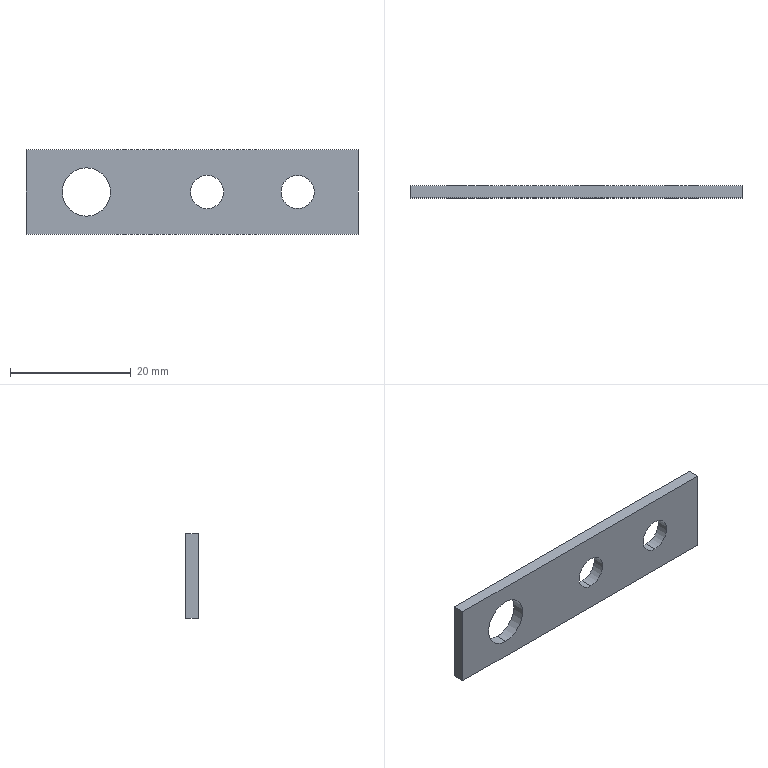Part | SolidWorks | features RefAxis 3, 3DProfileFeature 1, Extrusion 1 | 1 solid | 12 faces | box 55 x 2 x 14 mm | volume 1344 mm3 | cylinder 6 | plane 6 | commonest cylinder face diameters 5.5 x4 8 x2
STEP:
#1=CARTESIAN_POINT('',(0.,1.,-4.));
#2=VERTEX_POINT('',#1);
#3=CARTESIAN_POINT('',(0.,1.,4.));
#4=VERTEX_POINT('',#3);
#5=CARTESIAN_POINT('',(0.,1.,0.));
#6=DIRECTION('',(0.,1.,0.));
#7=DIRECTION('',(0.,0.,1.));
#8=AXIS2_PLACEMENT_3D('',#5,#6,#7);
#9=CIRCLE('',#8,4.);
#10=EDGE_CURVE('',#2,#4,#9,.T.);
#11=ORIENTED_EDGE('',*,*,#10,.T.);
#12=CARTESIAN_POINT('',(0.,-1.,4.));
#13=VERTEX_POINT('',#12);
#14=CARTESIAN_POINT('',(0.,1.,4.));
#15=DIRECTION('',(0.,-1.,0.));
#16=VECTOR('',#15,1000.);
#17=LINE('',#14,#16);
#18=EDGE_CURVE('',#4,#13,#17,.T.);
#19=ORIENTED_EDGE('',*,*,#18,.T.);
#20=CARTESIAN_POINT('',(0.,-1.,-4.));
#21=VERTEX_POINT('',#20);
#22=CARTESIAN_POINT('',(0.,-1.,0.));
#23=DIRECTION('',(0.,1.,0.));
#24=DIRECTION('',(0.,0.,1.));
#25=AXIS2_PLACEMENT_3D('',#22,#23,#24);
#26=CIRCLE('',#25,4.);
#27=EDGE_CURVE('',#21,#13,#26,.T.);
#28=ORIENTED_EDGE('',*,*,#27,.F.);
#29=CARTESIAN_POINT('',(0.,1.,-4.));
#30=DIRECTION('',(0.,-1.,0.));
#31=VECTOR('',#30,1000.);
#32=LINE('',#29,#31);
#33=EDGE_CURVE('',#2,#21,#32,.T.);
#34=ORIENTED_EDGE('',*,*,#33,.F.);
#35=EDGE_LOOP('',(#11,#19,#28,#34));
#36=FACE_OUTER_BOUND('',#35,.T.);
#37=CARTESIAN_POINT('',(0.,1.,0.));
#38=DIRECTION('',(0.,-1.,0.));
#39=DIRECTION('',(0.,0.,-1.));
#40=AXIS2_PLACEMENT_3D('',#37,#38,#39);
#41=CYLINDRICAL_SURFACE('',#40,4.);
#42=ADVANCED_FACE('',(#36),#41,.F.);
#43=CARTESIAN_POINT('',(20.,1.,-2.75));
#44=VERTEX_POINT('',#43);
#45=CARTESIAN_POINT('',(20.,1.,2.75));
#46=VERTEX_POINT('',#45);
#47=CARTESIAN_POINT('',(20.,1.,0.));
#48=DIRECTION('',(0.,1.,0.));
#49=DIRECTION('',(0.,0.,1.));
#50=AXIS2_PLACEMENT_3D('',#47,#48,#49);
#51=CIRCLE('',#50,2.75);
#52=EDGE_CURVE('',#44,#46,#51,.T.);
#53=ORIENTED_EDGE('',*,*,#52,.T.);
#54=CARTESIAN_POINT('',(20.,-1.,2.75));
#55=VERTEX_POINT('',#54);
#56=CARTESIAN_POINT('',(20.,1.,2.75));
#57=DIRECTION('',(0.,-1.,0.));
#58=VECTOR('',#57,1000.);
#59=LINE('',#56,#58);
#60=EDGE_CURVE('',#46,#55,#59,.T.);
#61=ORIENTED_EDGE('',*,*,#60,.T.);
#62=CARTESIAN_POINT('',(20.,-1.,-2.75));
#63=VERTEX_POINT('',#62);
#64=CARTESIAN_POINT('',(20.,-1.,0.));
#65=DIRECTION('',(0.,1.,0.));
#66=DIRECTION('',(0.,0.,1.));
#67=AXIS2_PLACEMENT_3D('',#64,#65,#66);
#68=CIRCLE('',#67,2.75);
#69=EDGE_CURVE('',#63,#55,#68,.T.);
#70=ORIENTED_EDGE('',*,*,#69,.F.);
#71=CARTESIAN_POINT('',(20.,1.,-2.75));
#72=DIRECTION('',(0.,-1.,0.));
#73=VECTOR('',#72,1000.);
#74=LINE('',#71,#73);
#75=EDGE_CURVE('',#44,#63,#74,.T.);
#76=ORIENTED_EDGE('',*,*,#75,.F.);
#77=EDGE_LOOP('',(#53,#61,#70,#76));
#78=FACE_OUTER_BOUND('',#77,.T.);
#79=CARTESIAN_POINT('',(20.,1.,0.));
#80=DIRECTION('',(0.,-1.,0.));
#81=DIRECTION('',(0.,0.,-1.));
#82=AXIS2_PLACEMENT_3D('',#79,#80,#81);
#83=CYLINDRICAL_SURFACE('',#82,2.75);
#84=ADVANCED_FACE('',(#78),#83,.F.);
#85=CARTESIAN_POINT('',(35.,1.,-2.75));
#86=VERTEX_POINT('',#85);
#87=CARTESIAN_POINT('',(35.,1.,2.75));
#88=VERTEX_POINT('',#87);
#89=CARTESIAN_POINT('',(35.,1.,0.));
#90=DIRECTION('',(0.,1.,0.));
#91=DIRECTION('',(0.,0.,1.));
#92=AXIS2_PLACEMENT_3D('',#89,#90,#91);
#93=CIRCLE('',#92,2.75);
#94=EDGE_CURVE('',#86,#88,#93,.T.);
#95=ORIENTED_EDGE('',*,*,#94,.T.);
#96=CARTESIAN_POINT('',(35.,-1.,2.75));
#97=VERTEX_POINT('',#96);
#98=CARTESIAN_POINT('',(35.,1.,2.75));
#99=DIRECTION('',(0.,-1.,0.));
#100=VECTOR('',#99,1000.);
#101=LINE('',#98,#100);
#102=EDGE_CURVE('',#88,#97,#101,.T.);
#103=ORIENTED_EDGE('',*,*,#102,.T.);
#104=CARTESIAN_POINT('',(35.,-1.,-2.75));
#105=VERTEX_POINT('',#104);
#106=CARTESIAN_POINT('',(35.,-1.,0.));
#107=DIRECTION('',(0.,1.,0.));
#108=DIRECTION('',(0.,0.,1.));
#109=AXIS2_PLACEMENT_3D('',#106,#107,#108);
#110=CIRCLE('',#109,2.75);
#111=EDGE_CURVE('',#105,#97,#110,.T.);
#112=ORIENTED_EDGE('',*,*,#111,.F.);
#113=CARTESIAN_POINT('',(35.,1.,-2.75));
#114=DIRECTION('',(0.,-1.,0.));
#115=VECTOR('',#114,1000.);
#116=LINE('',#113,#115);
#117=EDGE_CURVE('',#86,#105,#116,.T.);
#118=ORIENTED_EDGE('',*,*,#117,.F.);
#119=EDGE_LOOP('',(#95,#103,#112,#118));
#120=FACE_OUTER_BOUND('',#119,.T.);
#121=CARTESIAN_POINT('',(35.,1.,0.));
#122=DIRECTION('',(0.,-1.,0.));
#123=DIRECTION('',(0.,0.,-1.));
#124=AXIS2_PLACEMENT_3D('',#121,#122,#123);
#125=CYLINDRICAL_SURFACE('',#124,2.75);
#126=ADVANCED_FACE('',(#120),#125,.F.);
#127=ORIENTED_EDGE('',*,*,#52,.F.);
#128=CARTESIAN_POINT('',(20.,1.,0.));
#129=DIRECTION('',(0.,1.,0.));
#130=DIRECTION('',(0.,0.,1.));
#131=AXIS2_PLACEMENT_3D('',#128,#129,#130);
#132=CIRCLE('',#131,2.75);
#133=EDGE_CURVE('',#46,#44,#132,.T.);
#134=ORIENTED_EDGE('',*,*,#133,.F.);
#135=EDGE_LOOP('',(#127,#134));
#136=FACE_BOUND('',#135,.T.);
#137=CARTESIAN_POINT('',(45.,1.,-7.));
#138=VERTEX_POINT('',#137);
#139=CARTESIAN_POINT('',(-10.,1.,-7.));
#140=VERTEX_POINT('',#139);
#141=CARTESIAN_POINT('',(45.,1.,-7.));
#142=DIRECTION('',(-1.,0.,0.));
#143=VECTOR('',#142,1000.);
#144=LINE('',#141,#143);
#145=EDGE_CURVE('',#138,#140,#144,.T.);
#146=ORIENTED_EDGE('',*,*,#145,.T.);
#147=CARTESIAN_POINT('',(-10.,1.,7.));
#148=VERTEX_POINT('',#147);
#149=CARTESIAN_POINT('',(-10.,1.,-7.));
#150=DIRECTION('',(0.,0.,1.));
#151=VECTOR('',#150,1000.);
#152=LINE('',#149,#151);
#153=EDGE_CURVE('',#140,#148,#152,.T.);
#154=ORIENTED_EDGE('',*,*,#153,.T.);
#155=CARTESIAN_POINT('',(45.,1.,7.));
#156=VERTEX_POINT('',#155);
#157=CARTESIAN_POINT('',(-10.,1.,7.));
#158=DIRECTION('',(1.,0.,0.));
#159=VECTOR('',#158,1000.);
#160=LINE('',#157,#159);
#161=EDGE_CURVE('',#148,#156,#160,.T.);
#162=ORIENTED_EDGE('',*,*,#161,.T.);
#163=CARTESIAN_POINT('',(45.,1.,7.));
#164=DIRECTION('',(0.,0.,-1.));
#165=VECTOR('',#164,1000.);
#166=LINE('',#163,#165);
#167=EDGE_CURVE('',#156,#138,#166,.T.);
#168=ORIENTED_EDGE('',*,*,#167,.T.);
#169=EDGE_LOOP('',(#146,#154,#162,#168));
#170=FACE_OUTER_BOUND('',#169,.T.);
#171=ORIENTED_EDGE('',*,*,#94,.F.);
#172=CARTESIAN_POINT('',(35.,1.,0.));
#173=DIRECTION('',(0.,1.,0.));
#174=DIRECTION('',(0.,0.,1.));
#175=AXIS2_PLACEMENT_3D('',#172,#173,#174);
#176=CIRCLE('',#175,2.75);
#177=EDGE_CURVE('',#88,#86,#176,.T.);
#178=ORIENTED_EDGE('',*,*,#177,.F.);
#179=EDGE_LOOP('',(#171,#178));
#180=FACE_BOUND('',#179,.T.);
#181=ORIENTED_EDGE('',*,*,#10,.F.);
#182=CARTESIAN_POINT('',(0.,1.,0.));
#183=DIRECTION('',(0.,1.,0.));
#184=DIRECTION('',(0.,0.,1.));
#185=AXIS2_PLACEMENT_3D('',#182,#183,#184);
#186=CIRCLE('',#185,4.);
#187=EDGE_CURVE('',#4,#2,#186,.T.);
#188=ORIENTED_EDGE('',*,*,#187,.F.);
#189=EDGE_LOOP('',(#181,#188));
#190=FACE_BOUND('',#189,.T.);
#191=CARTESIAN_POINT('',(0.,1.,0.));
#192=DIRECTION('',(0.,1.,0.));
#193=DIRECTION('',(0.,0.,1.));
#194=AXIS2_PLACEMENT_3D('',#191,#192,#193);
#195=PLANE('',#194);
#196=ADVANCED_FACE('',(#136,#170,#180,#190),#195,.T.);
#197=CARTESIAN_POINT('',(45.,-1.,-7.));
#198=VERTEX_POINT('',#197);
#199=CARTESIAN_POINT('',(45.,1.,-7.));
#200=DIRECTION('',(0.,-1.,0.));
#201=VECTOR('',#200,1000.);
#202=LINE('',#199,#201);
#203=EDGE_CURVE('',#138,#198,#202,.T.);
#204=ORIENTED_EDGE('',*,*,#203,.T.);
#205=CARTESIAN_POINT('',(-10.,-1.,-7.));
#206=VERTEX_POINT('',#205);
#207=CARTESIAN_POINT('',(45.,-1.,-7.));
#208=DIRECTION('',(-1.,0.,0.));
#209=VECTOR('',#208,1000.);
#210=LINE('',#207,#209);
#211=EDGE_CURVE('',#198,#206,#210,.T.);
#212=ORIENTED_EDGE('',*,*,#211,.T.);
#213=CARTESIAN_POINT('',(-10.,1.,-7.));
#214=DIRECTION('',(0.,-1.,0.));
#215=VECTOR('',#214,1000.);
#216=LINE('',#213,#215);
#217=EDGE_CURVE('',#140,#206,#216,.T.);
#218=ORIENTED_EDGE('',*,*,#217,.F.);
#219=ORIENTED_EDGE('',*,*,#145,.F.);
#220=EDGE_LOOP('',(#204,#212,#218,#219));
#221=FACE_OUTER_BOUND('',#220,.T.);
#222=CARTESIAN_POINT('',(45.,1.,-7.));
#223=DIRECTION('',(0.,0.,1.));
#224=DIRECTION('',(1.,0.,0.));
#225=AXIS2_PLACEMENT_3D('',#222,#223,#224);
#226=PLANE('',#225);
#227=ADVANCED_FACE('',(#221),#226,.F.);
#228=ORIENTED_EDGE('',*,*,#217,.T.);
#229=CARTESIAN_POINT('',(-10.,-1.,7.));
#230=VERTEX_POINT('',#229);
#231=CARTESIAN_POINT('',(-10.,-1.,-7.));
#232=DIRECTION('',(0.,0.,1.));
#233=VECTOR('',#232,1000.);
#234=LINE('',#231,#233);
#235=EDGE_CURVE('',#206,#230,#234,.T.);
#236=ORIENTED_EDGE('',*,*,#235,.T.);
#237=CARTESIAN_POINT('',(-10.,1.,7.));
#238=DIRECTION('',(0.,-1.,0.));
#239=VECTOR('',#238,1000.);
#240=LINE('',#237,#239);
#241=EDGE_CURVE('',#148,#230,#240,.T.);
#242=ORIENTED_EDGE('',*,*,#241,.F.);
#243=ORIENTED_EDGE('',*,*,#153,.F.);
#244=EDGE_LOOP('',(#228,#236,#242,#243));
#245=FACE_OUTER_BOUND('',#244,.T.);
#246=CARTESIAN_POINT('',(-10.,1.,-7.));
#247=DIRECTION('',(1.,0.,0.));
#248=DIRECTION('',(0.,0.,-1.));
#249=AXIS2_PLACEMENT_3D('',#246,#247,#248);
#250=PLANE('',#249);
#251=ADVANCED_FACE('',(#245),#250,.F.);
#252=ORIENTED_EDGE('',*,*,#241,.T.);
#253=CARTESIAN_POINT('',(45.,-1.,7.));
#254=VERTEX_POINT('',#253);
#255=CARTESIAN_POINT('',(-10.,-1.,7.));
#256=DIRECTION('',(1.,0.,0.));
#257=VECTOR('',#256,1000.);
#258=LINE('',#255,#257);
#259=EDGE_CURVE('',#230,#254,#258,.T.);
#260=ORIENTED_EDGE('',*,*,#259,.T.);
#261=CARTESIAN_POINT('',(45.,1.,7.));
#262=DIRECTION('',(0.,-1.,0.));
#263=VECTOR('',#262,1000.);
#264=LINE('',#261,#263);
#265=EDGE_CURVE('',#156,#254,#264,.T.);
#266=ORIENTED_EDGE('',*,*,#265,.F.);
#267=ORIENTED_EDGE('',*,*,#161,.F.);
#268=EDGE_LOOP('',(#252,#260,#266,#267));
#269=FACE_OUTER_BOUND('',#268,.T.);
#270=CARTESIAN_POINT('',(-10.,1.,7.));
#271=DIRECTION('',(0.,0.,-1.));
#272=DIRECTION('',(-1.,0.,0.));
#273=AXIS2_PLACEMENT_3D('',#270,#271,#272);
#274=PLANE('',#273);
#275=ADVANCED_FACE('',(#269),#274,.F.);
#276=ORIENTED_EDGE('',*,*,#265,.T.);
#277=CARTESIAN_POINT('',(45.,-1.,7.));
#278=DIRECTION('',(0.,0.,-1.));
#279=VECTOR('',#278,1000.);
#280=LINE('',#277,#279);
#281=EDGE_CURVE('',#254,#198,#280,.T.);
#282=ORIENTED_EDGE('',*,*,#281,.T.);
#283=ORIENTED_EDGE('',*,*,#203,.F.);
#284=ORIENTED_EDGE('',*,*,#167,.F.);
#285=EDGE_LOOP('',(#276,#282,#283,#284));
#286=FACE_OUTER_BOUND('',#285,.T.);
#287=CARTESIAN_POINT('',(45.,1.,7.));
#288=DIRECTION('',(-1.,0.,0.));
#289=DIRECTION('',(0.,0.,1.));
#290=AXIS2_PLACEMENT_3D('',#287,#288,#289);
#291=PLANE('',#290);
#292=ADVANCED_FACE('',(#286),#291,.F.);
#293=ORIENTED_EDGE('',*,*,#102,.F.);
#294=ORIENTED_EDGE('',*,*,#177,.T.);
#295=ORIENTED_EDGE('',*,*,#117,.T.);
#296=CARTESIAN_POINT('',(35.,-1.,0.));
#297=DIRECTION('',(0.,1.,0.));
#298=DIRECTION('',(0.,0.,1.));
#299=AXIS2_PLACEMENT_3D('',#296,#297,#298);
#300=CIRCLE('',#299,2.75);
#301=EDGE_CURVE('',#97,#105,#300,.T.);
#302=ORIENTED_EDGE('',*,*,#301,.F.);
#303=EDGE_LOOP('',(#293,#294,#295,#302));
#304=FACE_OUTER_BOUND('',#303,.T.);
#305=CARTESIAN_POINT('',(35.,1.,0.));
#306=DIRECTION('',(0.,-1.,0.));
#307=DIRECTION('',(0.,0.,-1.));
#308=AXIS2_PLACEMENT_3D('',#305,#306,#307);
#309=CYLINDRICAL_SURFACE('',#308,2.75);
#310=ADVANCED_FACE('',(#304),#309,.F.);
#311=ORIENTED_EDGE('',*,*,#60,.F.);
#312=ORIENTED_EDGE('',*,*,#133,.T.);
#313=ORIENTED_EDGE('',*,*,#75,.T.);
#314=CARTESIAN_POINT('',(20.,-1.,0.));
#315=DIRECTION('',(0.,1.,0.));
#316=DIRECTION('',(0.,0.,1.));
#317=AXIS2_PLACEMENT_3D('',#314,#315,#316);
#318=CIRCLE('',#317,2.75);
#319=EDGE_CURVE('',#55,#63,#318,.T.);
#320=ORIENTED_EDGE('',*,*,#319,.F.);
#321=EDGE_LOOP('',(#311,#312,#313,#320));
#322=FACE_OUTER_BOUND('',#321,.T.);
#323=CARTESIAN_POINT('',(20.,1.,0.));
#324=DIRECTION('',(0.,-1.,0.));
#325=DIRECTION('',(0.,0.,-1.));
#326=AXIS2_PLACEMENT_3D('',#323,#324,#325);
#327=CYLINDRICAL_SURFACE('',#326,2.75);
#328=ADVANCED_FACE('',(#322),#327,.F.);
#329=ORIENTED_EDGE('',*,*,#18,.F.);
#330=ORIENTED_EDGE('',*,*,#187,.T.);
#331=ORIENTED_EDGE('',*,*,#33,.T.);
#332=CARTESIAN_POINT('',(0.,-1.,0.));
#333=DIRECTION('',(0.,1.,0.));
#334=DIRECTION('',(0.,0.,1.));
#335=AXIS2_PLACEMENT_3D('',#332,#333,#334);
#336=CIRCLE('',#335,4.);
#337=EDGE_CURVE('',#13,#21,#336,.T.);
#338=ORIENTED_EDGE('',*,*,#337,.F.);
#339=EDGE_LOOP('',(#329,#330,#331,#338));
#340=FACE_OUTER_BOUND('',#339,.T.);
#341=CARTESIAN_POINT('',(0.,1.,0.));
#342=DIRECTION('',(0.,-1.,0.));
#343=DIRECTION('',(0.,0.,-1.));
#344=AXIS2_PLACEMENT_3D('',#341,#342,#343);
#345=CYLINDRICAL_SURFACE('',#344,4.);
#346=ADVANCED_FACE('',(#340),#345,.F.);
#347=ORIENTED_EDGE('',*,*,#27,.T.);
#348=ORIENTED_EDGE('',*,*,#337,.T.);
#349=EDGE_LOOP('',(#347,#348));
#350=FACE_BOUND('',#349,.T.);
#351=ORIENTED_EDGE('',*,*,#69,.T.);
#352=ORIENTED_EDGE('',*,*,#319,.T.);
#353=EDGE_LOOP('',(#351,#352));
#354=FACE_BOUND('',#353,.T.);
#355=ORIENTED_EDGE('',*,*,#111,.T.);
#356=ORIENTED_EDGE('',*,*,#301,.T.);
#357=EDGE_LOOP('',(#355,#356));
#358=FACE_BOUND('',#357,.T.);
#359=ORIENTED_EDGE('',*,*,#211,.F.);
#360=ORIENTED_EDGE('',*,*,#281,.F.);
#361=ORIENTED_EDGE('',*,*,#259,.F.);
#362=ORIENTED_EDGE('',*,*,#235,.F.);
#363=EDGE_LOOP('',(#359,#360,#361,#362));
#364=FACE_OUTER_BOUND('',#363,.T.);
#365=CARTESIAN_POINT('',(0.,-1.,0.));
#366=DIRECTION('',(0.,1.,0.));
#367=DIRECTION('',(0.,0.,1.));
#368=AXIS2_PLACEMENT_3D('',#365,#366,#367);
#369=PLANE('',#368);
#370=ADVANCED_FACE('',(#350,#354,#358,#364),#369,.F.);
#371=CLOSED_SHELL('',(#42,#84,#126,#196,#227,#251,#275,#292,#310,#328,#346,#370));
#372=MANIFOLD_SOLID_BREP('',#371);
#373=CARTESIAN_POINT('',(0.,0.,0.));
#374=DIRECTION('',(0.,0.,1.));
#375=DIRECTION('',(1.,0.,0.));
#376=AXIS2_PLACEMENT_3D('',#373,#374,#375);
#377=(LENGTH_UNIT()NAMED_UNIT(*)SI_UNIT(.MILLI.,.METRE.));
#378=UNCERTAINTY_MEASURE_WITH_UNIT(LENGTH_MEASURE(0.00001),#377,'','');
#379=(NAMED_UNIT(*)PLANE_ANGLE_UNIT()SI_UNIT($,.RADIAN.));
#380=(NAMED_UNIT(*)SI_UNIT($,.STERADIAN.)SOLID_ANGLE_UNIT());
#381=(GEOMETRIC_REPRESENTATION_CONTEXT(3)GLOBAL_UNCERTAINTY_ASSIGNED_CONTEXT((#378))GLOBAL_UNIT_ASSIGNED_CONTEXT((#377,#379,#380))REPRESENTATION_CONTEXT('',''));
#382=ADVANCED_BREP_SHAPE_REPRESENTATION('',(#372,#376),#381);